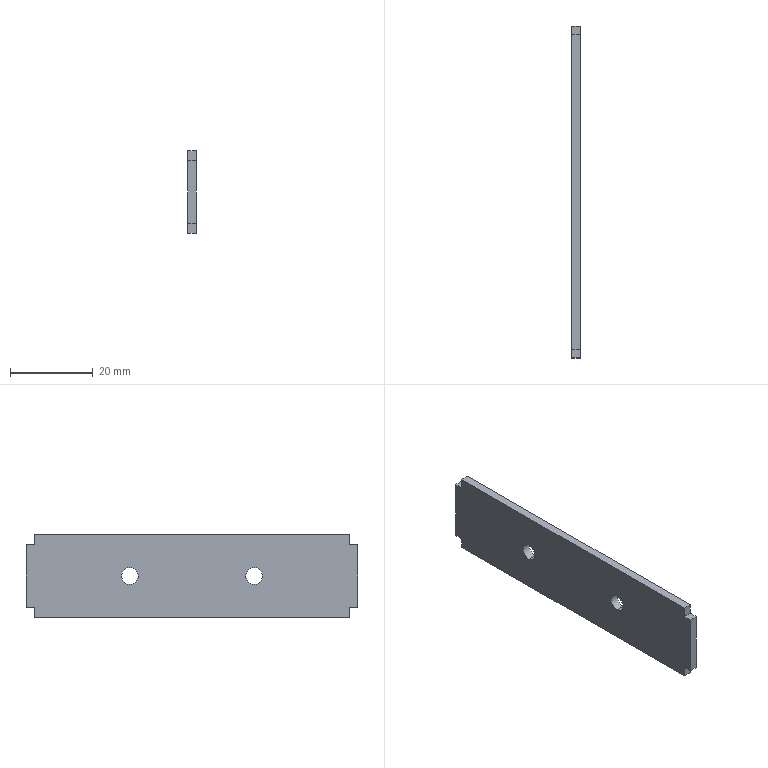Part | STEP file | 1 solid | 18 faces | box 2 x 80 x 20 mm | volume 3110 mm3 | plane 14 | cylinder 4 | commonest cylinder face diameters 4 x4
STEP:
#1=CARTESIAN_POINT('',(0.,0.,0.));
#2=DIRECTION('',(0.,0.,1.));
#3=DIRECTION('',(1.,0.,0.));
#4=AXIS2_PLACEMENT_3D('',#1,#2,#3);
#5=CARTESIAN_POINT('',(0.,-15.,-2.));
#6=VERTEX_POINT('',#5);
#7=CARTESIAN_POINT('',(2.,-15.,-2.));
#8=VERTEX_POINT('',#7);
#9=CARTESIAN_POINT('',(0.,-15.,-2.));
#10=DIRECTION('',(1.,0.,0.));
#11=VECTOR('',#10,1.);
#12=LINE('',#9,#11);
#13=CARTESIAN_POINT('',(0.,-15.,0.));
#14=DIRECTION('',(1.,0.,0.));
#15=DIRECTION('',(0.,0.,-1.));
#16=AXIS2_PLACEMENT_3D('',#13,#14,#15);
#17=CYLINDRICAL_SURFACE('',#16,2.);
#18=CARTESIAN_POINT('',(6.283,0.));
#19=DIRECTION('',(0.,1.));
#20=VECTOR('',#19,1.);
#21=LINE('',#18,#20);
#22=(GEOMETRIC_REPRESENTATION_CONTEXT(2)PARAMETRIC_REPRESENTATION_CONTEXT()REPRESENTATION_CONTEXT('',''));
#23=DEFINITIONAL_REPRESENTATION('',(#21),#22);
#24=PCURVE('',#17,#23);
#25=CARTESIAN_POINT('',(0.,-15.,0.));
#26=DIRECTION('',(1.,0.,0.));
#27=DIRECTION('',(0.,0.,-1.));
#28=AXIS2_PLACEMENT_3D('',#25,#26,#27);
#29=CYLINDRICAL_SURFACE('',#28,2.);
#30=CARTESIAN_POINT('',(0.,0.));
#31=DIRECTION('',(0.,1.));
#32=VECTOR('',#31,1.);
#33=LINE('',#30,#32);
#34=(GEOMETRIC_REPRESENTATION_CONTEXT(2)PARAMETRIC_REPRESENTATION_CONTEXT()REPRESENTATION_CONTEXT('',''));
#35=DEFINITIONAL_REPRESENTATION('',(#33),#34);
#36=PCURVE('',#29,#35);
#37=SURFACE_CURVE('',#12,(#24,#36),.PCURVE_S1.);
#38=EDGE_CURVE('',#6,#8,#37,.T.);
#39=ORIENTED_EDGE('',*,*,#38,.T.);
#40=CARTESIAN_POINT('',(2.,-15.,2.));
#41=VERTEX_POINT('',#40);
#42=CARTESIAN_POINT('',(2.,-15.,0.));
#43=DIRECTION('',(-1.,0.,0.));
#44=DIRECTION('',(0.,0.,-1.));
#45=AXIS2_PLACEMENT_3D('',#42,#43,#44);
#46=CIRCLE('',#45,2.);
#47=CARTESIAN_POINT('',(6.283,2.));
#48=DIRECTION('',(-1.,0.));
#49=VECTOR('',#48,1.);
#50=LINE('',#47,#49);
#51=(GEOMETRIC_REPRESENTATION_CONTEXT(2)PARAMETRIC_REPRESENTATION_CONTEXT()REPRESENTATION_CONTEXT('',''));
#52=DEFINITIONAL_REPRESENTATION('',(#50),#51);
#53=PCURVE('',#17,#52);
#54=CARTESIAN_POINT('',(2.,-19.917,0.));
#55=DIRECTION('',(1.,0.,0.));
#56=DIRECTION('',(0.,0.,-1.));
#57=AXIS2_PLACEMENT_3D('',#54,#55,#56);
#58=PLANE('',#57);
#59=CARTESIAN_POINT('',(2.,4.917));
#60=CARTESIAN_POINT('',(2.,1.453));
#61=CARTESIAN_POINT('',(-1.,3.185));
#62=CARTESIAN_POINT('',(-4.,4.917));
#63=CARTESIAN_POINT('',(-1.,6.649));
#64=CARTESIAN_POINT('',(2.,8.381));
#65=CARTESIAN_POINT('',(2.,4.917));
#66=(BOUNDED_CURVE()B_SPLINE_CURVE(2,(#59,#60,#61,#62,#63,#64,#65),.UNSPECIFIED.,.T.,.F.)B_SPLINE_CURVE_WITH_KNOTS((1,2,2,2,2,1),(-2.094,0.,2.094,4.189,6.283,8.378),.UNSPECIFIED.)CURVE()GEOMETRIC_REPRESENTATION_ITEM()RATIONAL_B_SPLINE_CURVE((1.,0.5,1.,0.5,1.,0.5,1.))REPRESENTATION_ITEM(''));
#67=(GEOMETRIC_REPRESENTATION_CONTEXT(2)PARAMETRIC_REPRESENTATION_CONTEXT()REPRESENTATION_CONTEXT('',''));
#68=DEFINITIONAL_REPRESENTATION('',(#66),#67);
#69=PCURVE('',#58,#68);
#70=SURFACE_CURVE('',#46,(#53,#69),.PCURVE_S1.);
#71=EDGE_CURVE('',#8,#41,#70,.T.);
#72=ORIENTED_EDGE('',*,*,#71,.T.);
#73=CARTESIAN_POINT('',(0.,-15.,2.));
#74=VERTEX_POINT('',#73);
#75=CARTESIAN_POINT('',(0.,-15.,2.));
#76=DIRECTION('',(1.,0.,0.));
#77=VECTOR('',#76,1.);
#78=LINE('',#75,#77);
#79=CARTESIAN_POINT('',(3.142,0.));
#80=DIRECTION('',(0.,1.));
#81=VECTOR('',#80,1.);
#82=LINE('',#79,#81);
#83=(GEOMETRIC_REPRESENTATION_CONTEXT(2)PARAMETRIC_REPRESENTATION_CONTEXT()REPRESENTATION_CONTEXT('',''));
#84=DEFINITIONAL_REPRESENTATION('',(#82),#83);
#85=PCURVE('',#17,#84);
#86=CARTESIAN_POINT('',(3.142,0.));
#87=DIRECTION('',(0.,1.));
#88=VECTOR('',#87,1.);
#89=LINE('',#86,#88);
#90=(GEOMETRIC_REPRESENTATION_CONTEXT(2)PARAMETRIC_REPRESENTATION_CONTEXT()REPRESENTATION_CONTEXT('',''));
#91=DEFINITIONAL_REPRESENTATION('',(#89),#90);
#92=PCURVE('',#29,#91);
#93=SURFACE_CURVE('',#78,(#85,#92),.PCURVE_S1.);
#94=EDGE_CURVE('',#74,#41,#93,.T.);
#95=ORIENTED_EDGE('',*,*,#94,.F.);
#96=CARTESIAN_POINT('',(0.,-15.,0.));
#97=DIRECTION('',(1.,0.,0.));
#98=DIRECTION('',(0.,0.,-1.));
#99=AXIS2_PLACEMENT_3D('',#96,#97,#98);
#100=CIRCLE('',#99,2.);
#101=CARTESIAN_POINT('',(0.,0.));
#102=DIRECTION('',(1.,0.));
#103=VECTOR('',#102,1.);
#104=LINE('',#101,#103);
#105=(GEOMETRIC_REPRESENTATION_CONTEXT(2)PARAMETRIC_REPRESENTATION_CONTEXT()REPRESENTATION_CONTEXT('',''));
#106=DEFINITIONAL_REPRESENTATION('',(#104),#105);
#107=PCURVE('',#17,#106);
#108=CARTESIAN_POINT('',(0.,-19.917,0.));
#109=DIRECTION('',(1.,0.,0.));
#110=DIRECTION('',(0.,0.,-1.));
#111=AXIS2_PLACEMENT_3D('',#108,#109,#110);
#112=PLANE('',#111);
#113=CARTESIAN_POINT('',(0.,4.917));
#114=DIRECTION('',(1.,0.));
#115=AXIS2_PLACEMENT_2D('',#113,#114);
#116=CIRCLE('',#115,2.);
#117=(GEOMETRIC_REPRESENTATION_CONTEXT(2)PARAMETRIC_REPRESENTATION_CONTEXT()REPRESENTATION_CONTEXT('',''));
#118=DEFINITIONAL_REPRESENTATION('',(#116),#117);
#119=PCURVE('',#112,#118);
#120=SURFACE_CURVE('',#100,(#107,#119),.PCURVE_S1.);
#121=EDGE_CURVE('',#74,#6,#120,.T.);
#122=ORIENTED_EDGE('',*,*,#121,.T.);
#123=EDGE_LOOP('',(#39,#72,#95,#122));
#124=FACE_BOUND('',#123,.F.);
#125=ADVANCED_FACE('',(#124),#17,.F.);
#126=CARTESIAN_POINT('',(0.,15.,-2.));
#127=VERTEX_POINT('',#126);
#128=CARTESIAN_POINT('',(2.,15.,-2.));
#129=VERTEX_POINT('',#128);
#130=CARTESIAN_POINT('',(0.,15.,-2.));
#131=DIRECTION('',(1.,0.,0.));
#132=VECTOR('',#131,1.);
#133=LINE('',#130,#132);
#134=CARTESIAN_POINT('',(0.,15.,0.));
#135=DIRECTION('',(1.,0.,0.));
#136=DIRECTION('',(0.,0.,-1.));
#137=AXIS2_PLACEMENT_3D('',#134,#135,#136);
#138=CYLINDRICAL_SURFACE('',#137,2.);
#139=CARTESIAN_POINT('',(6.283,0.));
#140=DIRECTION('',(0.,1.));
#141=VECTOR('',#140,1.);
#142=LINE('',#139,#141);
#143=(GEOMETRIC_REPRESENTATION_CONTEXT(2)PARAMETRIC_REPRESENTATION_CONTEXT()REPRESENTATION_CONTEXT('',''));
#144=DEFINITIONAL_REPRESENTATION('',(#142),#143);
#145=PCURVE('',#138,#144);
#146=CARTESIAN_POINT('',(0.,15.,0.));
#147=DIRECTION('',(1.,0.,0.));
#148=DIRECTION('',(0.,0.,-1.));
#149=AXIS2_PLACEMENT_3D('',#146,#147,#148);
#150=CYLINDRICAL_SURFACE('',#149,2.);
#151=CARTESIAN_POINT('',(0.,0.));
#152=DIRECTION('',(0.,1.));
#153=VECTOR('',#152,1.);
#154=LINE('',#151,#153);
#155=(GEOMETRIC_REPRESENTATION_CONTEXT(2)PARAMETRIC_REPRESENTATION_CONTEXT()REPRESENTATION_CONTEXT('',''));
#156=DEFINITIONAL_REPRESENTATION('',(#154),#155);
#157=PCURVE('',#150,#156);
#158=SURFACE_CURVE('',#133,(#145,#157),.PCURVE_S1.);
#159=EDGE_CURVE('',#127,#129,#158,.T.);
#160=ORIENTED_EDGE('',*,*,#159,.T.);
#161=CARTESIAN_POINT('',(2.,15.,2.));
#162=VERTEX_POINT('',#161);
#163=CARTESIAN_POINT('',(2.,15.,0.));
#164=DIRECTION('',(-1.,0.,0.));
#165=DIRECTION('',(0.,0.,-1.));
#166=AXIS2_PLACEMENT_3D('',#163,#164,#165);
#167=CIRCLE('',#166,2.);
#168=CARTESIAN_POINT('',(6.283,2.));
#169=DIRECTION('',(-1.,0.));
#170=VECTOR('',#169,1.);
#171=LINE('',#168,#170);
#172=(GEOMETRIC_REPRESENTATION_CONTEXT(2)PARAMETRIC_REPRESENTATION_CONTEXT()REPRESENTATION_CONTEXT('',''));
#173=DEFINITIONAL_REPRESENTATION('',(#171),#172);
#174=PCURVE('',#138,#173);
#175=CARTESIAN_POINT('',(2.,34.917));
#176=CARTESIAN_POINT('',(2.,31.453));
#177=CARTESIAN_POINT('',(-1.,33.185));
#178=CARTESIAN_POINT('',(-4.,34.917));
#179=CARTESIAN_POINT('',(-1.,36.649));
#180=CARTESIAN_POINT('',(2.,38.381));
#181=CARTESIAN_POINT('',(2.,34.917));
#182=(BOUNDED_CURVE()B_SPLINE_CURVE(2,(#175,#176,#177,#178,#179,#180,#181),.UNSPECIFIED.,.T.,.F.)B_SPLINE_CURVE_WITH_KNOTS((1,2,2,2,2,1),(-2.094,0.,2.094,4.189,6.283,8.378),.UNSPECIFIED.)CURVE()GEOMETRIC_REPRESENTATION_ITEM()RATIONAL_B_SPLINE_CURVE((1.,0.5,1.,0.5,1.,0.5,1.))REPRESENTATION_ITEM(''));
#183=(GEOMETRIC_REPRESENTATION_CONTEXT(2)PARAMETRIC_REPRESENTATION_CONTEXT()REPRESENTATION_CONTEXT('',''));
#184=DEFINITIONAL_REPRESENTATION('',(#182),#183);
#185=PCURVE('',#58,#184);
#186=SURFACE_CURVE('',#167,(#174,#185),.PCURVE_S1.);
#187=EDGE_CURVE('',#129,#162,#186,.T.);
#188=ORIENTED_EDGE('',*,*,#187,.T.);
#189=CARTESIAN_POINT('',(0.,15.,2.));
#190=VERTEX_POINT('',#189);
#191=CARTESIAN_POINT('',(0.,15.,2.));
#192=DIRECTION('',(1.,0.,0.));
#193=VECTOR('',#192,1.);
#194=LINE('',#191,#193);
#195=CARTESIAN_POINT('',(3.142,0.));
#196=DIRECTION('',(0.,1.));
#197=VECTOR('',#196,1.);
#198=LINE('',#195,#197);
#199=(GEOMETRIC_REPRESENTATION_CONTEXT(2)PARAMETRIC_REPRESENTATION_CONTEXT()REPRESENTATION_CONTEXT('',''));
#200=DEFINITIONAL_REPRESENTATION('',(#198),#199);
#201=PCURVE('',#138,#200);
#202=CARTESIAN_POINT('',(3.142,0.));
#203=DIRECTION('',(0.,1.));
#204=VECTOR('',#203,1.);
#205=LINE('',#202,#204);
#206=(GEOMETRIC_REPRESENTATION_CONTEXT(2)PARAMETRIC_REPRESENTATION_CONTEXT()REPRESENTATION_CONTEXT('',''));
#207=DEFINITIONAL_REPRESENTATION('',(#205),#206);
#208=PCURVE('',#150,#207);
#209=SURFACE_CURVE('',#194,(#201,#208),.PCURVE_S1.);
#210=EDGE_CURVE('',#190,#162,#209,.T.);
#211=ORIENTED_EDGE('',*,*,#210,.F.);
#212=CARTESIAN_POINT('',(0.,15.,0.));
#213=DIRECTION('',(1.,0.,0.));
#214=DIRECTION('',(0.,0.,-1.));
#215=AXIS2_PLACEMENT_3D('',#212,#213,#214);
#216=CIRCLE('',#215,2.);
#217=CARTESIAN_POINT('',(0.,0.));
#218=DIRECTION('',(1.,0.));
#219=VECTOR('',#218,1.);
#220=LINE('',#217,#219);
#221=(GEOMETRIC_REPRESENTATION_CONTEXT(2)PARAMETRIC_REPRESENTATION_CONTEXT()REPRESENTATION_CONTEXT('',''));
#222=DEFINITIONAL_REPRESENTATION('',(#220),#221);
#223=PCURVE('',#138,#222);
#224=CARTESIAN_POINT('',(0.,34.917));
#225=DIRECTION('',(1.,0.));
#226=AXIS2_PLACEMENT_2D('',#224,#225);
#227=CIRCLE('',#226,2.);
#228=(GEOMETRIC_REPRESENTATION_CONTEXT(2)PARAMETRIC_REPRESENTATION_CONTEXT()REPRESENTATION_CONTEXT('',''));
#229=DEFINITIONAL_REPRESENTATION('',(#227),#228);
#230=PCURVE('',#112,#229);
#231=SURFACE_CURVE('',#216,(#223,#230),.PCURVE_S1.);
#232=EDGE_CURVE('',#190,#127,#231,.T.);
#233=ORIENTED_EDGE('',*,*,#232,.T.);
#234=EDGE_LOOP('',(#160,#188,#211,#233));
#235=FACE_BOUND('',#234,.F.);
#236=ADVANCED_FACE('',(#235),#138,.F.);
#237=CARTESIAN_POINT('',(2.,40.,7.5));
#238=VERTEX_POINT('',#237);
#239=CARTESIAN_POINT('',(2.,38.,7.5));
#240=VERTEX_POINT('',#239);
#241=CARTESIAN_POINT('',(2.,-19.917,7.5));
#242=DIRECTION('',(0.,-1.,0.));
#243=VECTOR('',#242,1.);
#244=LINE('',#241,#243);
#245=CARTESIAN_POINT('',(-7.5,0.));
#246=DIRECTION('',(0.,-1.));
#247=VECTOR('',#246,1.);
#248=LINE('',#245,#247);
#249=(GEOMETRIC_REPRESENTATION_CONTEXT(2)PARAMETRIC_REPRESENTATION_CONTEXT()REPRESENTATION_CONTEXT('',''));
#250=DEFINITIONAL_REPRESENTATION('',(#248),#249);
#251=PCURVE('',#58,#250);
#252=CARTESIAN_POINT('',(0.,40.,7.5));
#253=DIRECTION('',(0.,0.,1.));
#254=DIRECTION('',(0.,-1.,0.));
#255=AXIS2_PLACEMENT_3D('',#252,#253,#254);
#256=PLANE('',#255);
#257=CARTESIAN_POINT('',(59.917,2.));
#258=DIRECTION('',(1.,0.));
#259=VECTOR('',#258,1.);
#260=LINE('',#257,#259);
#261=(GEOMETRIC_REPRESENTATION_CONTEXT(2)PARAMETRIC_REPRESENTATION_CONTEXT()REPRESENTATION_CONTEXT('',''));
#262=DEFINITIONAL_REPRESENTATION('',(#260),#261);
#263=PCURVE('',#256,#262);
#264=SURFACE_CURVE('',#244,(#251,#263),.PCURVE_S1.);
#265=EDGE_CURVE('',#238,#240,#264,.T.);
#266=ORIENTED_EDGE('',*,*,#265,.T.);
#267=CARTESIAN_POINT('',(2.,38.,10.));
#268=VERTEX_POINT('',#267);
#269=CARTESIAN_POINT('',(2.,38.,0.));
#270=DIRECTION('',(0.,0.,1.));
#271=VECTOR('',#270,1.);
#272=LINE('',#269,#271);
#273=CARTESIAN_POINT('',(0.,57.917));
#274=DIRECTION('',(-1.,0.));
#275=VECTOR('',#274,1.);
#276=LINE('',#273,#275);
#277=(GEOMETRIC_REPRESENTATION_CONTEXT(2)PARAMETRIC_REPRESENTATION_CONTEXT()REPRESENTATION_CONTEXT('',''));
#278=DEFINITIONAL_REPRESENTATION('',(#276),#277);
#279=PCURVE('',#58,#278);
#280=CARTESIAN_POINT('',(0.,38.,7.5));
#281=DIRECTION('',(0.,1.,0.));
#282=DIRECTION('',(0.,0.,1.));
#283=AXIS2_PLACEMENT_3D('',#280,#281,#282);
#284=PLANE('',#283);
#285=CARTESIAN_POINT('',(-7.5,2.));
#286=DIRECTION('',(1.,0.));
#287=VECTOR('',#286,1.);
#288=LINE('',#285,#287);
#289=(GEOMETRIC_REPRESENTATION_CONTEXT(2)PARAMETRIC_REPRESENTATION_CONTEXT()REPRESENTATION_CONTEXT('',''));
#290=DEFINITIONAL_REPRESENTATION('',(#288),#289);
#291=PCURVE('',#284,#290);
#292=SURFACE_CURVE('',#272,(#279,#291),.PCURVE_S1.);
#293=EDGE_CURVE('',#240,#268,#292,.T.);
#294=ORIENTED_EDGE('',*,*,#293,.T.);
#295=CARTESIAN_POINT('',(2.,-38.,10.));
#296=VERTEX_POINT('',#295);
#297=CARTESIAN_POINT('',(2.,-19.917,10.));
#298=DIRECTION('',(0.,-1.,0.));
#299=VECTOR('',#298,1.);
#300=LINE('',#297,#299);
#301=CARTESIAN_POINT('',(-10.,0.));
#302=DIRECTION('',(0.,-1.));
#303=VECTOR('',#302,1.);
#304=LINE('',#301,#303);
#305=(GEOMETRIC_REPRESENTATION_CONTEXT(2)PARAMETRIC_REPRESENTATION_CONTEXT()REPRESENTATION_CONTEXT('',''));
#306=DEFINITIONAL_REPRESENTATION('',(#304),#305);
#307=PCURVE('',#58,#306);
#308=CARTESIAN_POINT('',(0.,0.,10.));
#309=DIRECTION('',(0.,0.,1.));
#310=DIRECTION('',(1.,0.,0.));
#311=AXIS2_PLACEMENT_3D('',#308,#309,#310);
#312=PLANE('',#311);
#313=CARTESIAN_POINT('',(2.,-19.917));
#314=DIRECTION('',(0.,-1.));
#315=VECTOR('',#314,1.);
#316=LINE('',#313,#315);
#317=(GEOMETRIC_REPRESENTATION_CONTEXT(2)PARAMETRIC_REPRESENTATION_CONTEXT()REPRESENTATION_CONTEXT('',''));
#318=DEFINITIONAL_REPRESENTATION('',(#316),#317);
#319=PCURVE('',#312,#318);
#320=SURFACE_CURVE('',#300,(#307,#319),.PCURVE_S1.);
#321=EDGE_CURVE('',#268,#296,#320,.T.);
#322=ORIENTED_EDGE('',*,*,#321,.T.);
#323=CARTESIAN_POINT('',(2.,-38.,7.5));
#324=VERTEX_POINT('',#323);
#325=CARTESIAN_POINT('',(2.,-38.,0.));
#326=DIRECTION('',(0.,0.,-1.));
#327=VECTOR('',#326,1.);
#328=LINE('',#325,#327);
#329=CARTESIAN_POINT('',(0.,-18.083));
#330=DIRECTION('',(1.,0.));
#331=VECTOR('',#330,1.);
#332=LINE('',#329,#331);
#333=(GEOMETRIC_REPRESENTATION_CONTEXT(2)PARAMETRIC_REPRESENTATION_CONTEXT()REPRESENTATION_CONTEXT('',''));
#334=DEFINITIONAL_REPRESENTATION('',(#332),#333);
#335=PCURVE('',#58,#334);
#336=CARTESIAN_POINT('',(0.,-38.,10.));
#337=DIRECTION('',(0.,-1.,0.));
#338=DIRECTION('',(0.,0.,-1.));
#339=AXIS2_PLACEMENT_3D('',#336,#337,#338);
#340=PLANE('',#339);
#341=CARTESIAN_POINT('',(10.,2.));
#342=DIRECTION('',(1.,0.));
#343=VECTOR('',#342,1.);
#344=LINE('',#341,#343);
#345=(GEOMETRIC_REPRESENTATION_CONTEXT(2)PARAMETRIC_REPRESENTATION_CONTEXT()REPRESENTATION_CONTEXT('',''));
#346=DEFINITIONAL_REPRESENTATION('',(#344),#345);
#347=PCURVE('',#340,#346);
#348=SURFACE_CURVE('',#328,(#335,#347),.PCURVE_S1.);
#349=EDGE_CURVE('',#296,#324,#348,.T.);
#350=ORIENTED_EDGE('',*,*,#349,.T.);
#351=CARTESIAN_POINT('',(2.,-40.,7.5));
#352=VERTEX_POINT('',#351);
#353=CARTESIAN_POINT('',(2.,-19.917,7.5));
#354=DIRECTION('',(0.,-1.,0.));
#355=VECTOR('',#354,1.);
#356=LINE('',#353,#355);
#357=CARTESIAN_POINT('',(-7.5,0.));
#358=DIRECTION('',(0.,-1.));
#359=VECTOR('',#358,1.);
#360=LINE('',#357,#359);
#361=(GEOMETRIC_REPRESENTATION_CONTEXT(2)PARAMETRIC_REPRESENTATION_CONTEXT()REPRESENTATION_CONTEXT('',''));
#362=DEFINITIONAL_REPRESENTATION('',(#360),#361);
#363=PCURVE('',#58,#362);
#364=CARTESIAN_POINT('',(0.,-38.,7.5));
#365=DIRECTION('',(0.,0.,1.));
#366=DIRECTION('',(1.,0.,0.));
#367=AXIS2_PLACEMENT_3D('',#364,#365,#366);
#368=PLANE('',#367);
#369=CARTESIAN_POINT('',(2.,18.083));
#370=DIRECTION('',(0.,-1.));
#371=VECTOR('',#370,1.);
#372=LINE('',#369,#371);
#373=(GEOMETRIC_REPRESENTATION_CONTEXT(2)PARAMETRIC_REPRESENTATION_CONTEXT()REPRESENTATION_CONTEXT('',''));
#374=DEFINITIONAL_REPRESENTATION('',(#372),#373);
#375=PCURVE('',#368,#374);
#376=SURFACE_CURVE('',#356,(#363,#375),.PCURVE_S1.);
#377=EDGE_CURVE('',#324,#352,#376,.T.);
#378=ORIENTED_EDGE('',*,*,#377,.T.);
#379=CARTESIAN_POINT('',(2.,-40.,-7.5));
#380=VERTEX_POINT('',#379);
#381=CARTESIAN_POINT('',(2.,-40.,0.));
#382=DIRECTION('',(0.,0.,-1.));
#383=VECTOR('',#382,1.);
#384=LINE('',#381,#383);
#385=CARTESIAN_POINT('',(0.,-20.083));
#386=DIRECTION('',(1.,0.));
#387=VECTOR('',#386,1.);
#388=LINE('',#385,#387);
#389=(GEOMETRIC_REPRESENTATION_CONTEXT(2)PARAMETRIC_REPRESENTATION_CONTEXT()REPRESENTATION_CONTEXT('',''));
#390=DEFINITIONAL_REPRESENTATION('',(#388),#389);
#391=PCURVE('',#58,#390);
#392=CARTESIAN_POINT('',(0.,-40.,7.5));
#393=DIRECTION('',(0.,-1.,0.));
#394=DIRECTION('',(0.,0.,-1.));
#395=AXIS2_PLACEMENT_3D('',#392,#393,#394);
#396=PLANE('',#395);
#397=CARTESIAN_POINT('',(7.5,2.));
#398=DIRECTION('',(1.,0.));
#399=VECTOR('',#398,1.);
#400=LINE('',#397,#399);
#401=(GEOMETRIC_REPRESENTATION_CONTEXT(2)PARAMETRIC_REPRESENTATION_CONTEXT()REPRESENTATION_CONTEXT('',''));
#402=DEFINITIONAL_REPRESENTATION('',(#400),#401);
#403=PCURVE('',#396,#402);
#404=SURFACE_CURVE('',#384,(#391,#403),.PCURVE_S1.);
#405=EDGE_CURVE('',#352,#380,#404,.T.);
#406=ORIENTED_EDGE('',*,*,#405,.T.);
#407=CARTESIAN_POINT('',(2.,-38.,-7.5));
#408=VERTEX_POINT('',#407);
#409=CARTESIAN_POINT('',(2.,-19.917,-7.5));
#410=DIRECTION('',(0.,1.,0.));
#411=VECTOR('',#410,1.);
#412=LINE('',#409,#411);
#413=CARTESIAN_POINT('',(7.5,0.));
#414=DIRECTION('',(0.,1.));
#415=VECTOR('',#414,1.);
#416=LINE('',#413,#415);
#417=(GEOMETRIC_REPRESENTATION_CONTEXT(2)PARAMETRIC_REPRESENTATION_CONTEXT()REPRESENTATION_CONTEXT('',''));
#418=DEFINITIONAL_REPRESENTATION('',(#416),#417);
#419=PCURVE('',#58,#418);
#420=CARTESIAN_POINT('',(0.,-40.,-7.5));
#421=DIRECTION('',(0.,0.,-1.));
#422=DIRECTION('',(-1.,0.,0.));
#423=AXIS2_PLACEMENT_3D('',#420,#421,#422);
#424=PLANE('',#423);
#425=CARTESIAN_POINT('',(-2.,20.083));
#426=DIRECTION('',(0.,1.));
#427=VECTOR('',#426,1.);
#428=LINE('',#425,#427);
#429=(GEOMETRIC_REPRESENTATION_CONTEXT(2)PARAMETRIC_REPRESENTATION_CONTEXT()REPRESENTATION_CONTEXT('',''));
#430=DEFINITIONAL_REPRESENTATION('',(#428),#429);
#431=PCURVE('',#424,#430);
#432=SURFACE_CURVE('',#412,(#419,#431),.PCURVE_S1.);
#433=EDGE_CURVE('',#380,#408,#432,.T.);
#434=ORIENTED_EDGE('',*,*,#433,.T.);
#435=CARTESIAN_POINT('',(2.,-38.,-10.));
#436=VERTEX_POINT('',#435);
#437=CARTESIAN_POINT('',(2.,-38.,0.));
#438=DIRECTION('',(0.,0.,-1.));
#439=VECTOR('',#438,1.);
#440=LINE('',#437,#439);
#441=CARTESIAN_POINT('',(0.,-18.083));
#442=DIRECTION('',(1.,0.));
#443=VECTOR('',#442,1.);
#444=LINE('',#441,#443);
#445=(GEOMETRIC_REPRESENTATION_CONTEXT(2)PARAMETRIC_REPRESENTATION_CONTEXT()REPRESENTATION_CONTEXT('',''));
#446=DEFINITIONAL_REPRESENTATION('',(#444),#445);
#447=PCURVE('',#58,#446);
#448=CARTESIAN_POINT('',(0.,-38.,-7.5));
#449=DIRECTION('',(0.,-1.,0.));
#450=DIRECTION('',(0.,0.,-1.));
#451=AXIS2_PLACEMENT_3D('',#448,#449,#450);
#452=PLANE('',#451);
#453=CARTESIAN_POINT('',(-7.5,2.));
#454=DIRECTION('',(1.,0.));
#455=VECTOR('',#454,1.);
#456=LINE('',#453,#455);
#457=(GEOMETRIC_REPRESENTATION_CONTEXT(2)PARAMETRIC_REPRESENTATION_CONTEXT()REPRESENTATION_CONTEXT('',''));
#458=DEFINITIONAL_REPRESENTATION('',(#456),#457);
#459=PCURVE('',#452,#458);
#460=SURFACE_CURVE('',#440,(#447,#459),.PCURVE_S1.);
#461=EDGE_CURVE('',#408,#436,#460,.T.);
#462=ORIENTED_EDGE('',*,*,#461,.T.);
#463=CARTESIAN_POINT('',(2.,38.,-10.));
#464=VERTEX_POINT('',#463);
#465=CARTESIAN_POINT('',(2.,-19.917,-10.));
#466=DIRECTION('',(0.,1.,0.));
#467=VECTOR('',#466,1.);
#468=LINE('',#465,#467);
#469=CARTESIAN_POINT('',(10.,0.));
#470=DIRECTION('',(0.,1.));
#471=VECTOR('',#470,1.);
#472=LINE('',#469,#471);
#473=(GEOMETRIC_REPRESENTATION_CONTEXT(2)PARAMETRIC_REPRESENTATION_CONTEXT()REPRESENTATION_CONTEXT('',''));
#474=DEFINITIONAL_REPRESENTATION('',(#472),#473);
#475=PCURVE('',#58,#474);
#476=CARTESIAN_POINT('',(0.,-38.,-10.));
#477=DIRECTION('',(0.,0.,-1.));
#478=DIRECTION('',(-1.,0.,0.));
#479=AXIS2_PLACEMENT_3D('',#476,#477,#478);
#480=PLANE('',#479);
#481=CARTESIAN_POINT('',(-2.,18.083));
#482=DIRECTION('',(0.,1.));
#483=VECTOR('',#482,1.);
#484=LINE('',#481,#483);
#485=(GEOMETRIC_REPRESENTATION_CONTEXT(2)PARAMETRIC_REPRESENTATION_CONTEXT()REPRESENTATION_CONTEXT('',''));
#486=DEFINITIONAL_REPRESENTATION('',(#484),#485);
#487=PCURVE('',#480,#486);
#488=SURFACE_CURVE('',#468,(#475,#487),.PCURVE_S1.);
#489=EDGE_CURVE('',#436,#464,#488,.T.);
#490=ORIENTED_EDGE('',*,*,#489,.T.);
#491=CARTESIAN_POINT('',(2.,38.,-7.5));
#492=VERTEX_POINT('',#491);
#493=CARTESIAN_POINT('',(2.,38.,0.));
#494=DIRECTION('',(0.,0.,1.));
#495=VECTOR('',#494,1.);
#496=LINE('',#493,#495);
#497=CARTESIAN_POINT('',(0.,57.917));
#498=DIRECTION('',(-1.,0.));
#499=VECTOR('',#498,1.);
#500=LINE('',#497,#499);
#501=(GEOMETRIC_REPRESENTATION_CONTEXT(2)PARAMETRIC_REPRESENTATION_CONTEXT()REPRESENTATION_CONTEXT('',''));
#502=DEFINITIONAL_REPRESENTATION('',(#500),#501);
#503=PCURVE('',#58,#502);
#504=CARTESIAN_POINT('',(0.,38.,-10.));
#505=DIRECTION('',(0.,1.,0.));
#506=DIRECTION('',(0.,0.,1.));
#507=AXIS2_PLACEMENT_3D('',#504,#505,#506);
#508=PLANE('',#507);
#509=CARTESIAN_POINT('',(10.,2.));
#510=DIRECTION('',(1.,0.));
#511=VECTOR('',#510,1.);
#512=LINE('',#509,#511);
#513=(GEOMETRIC_REPRESENTATION_CONTEXT(2)PARAMETRIC_REPRESENTATION_CONTEXT()REPRESENTATION_CONTEXT('',''));
#514=DEFINITIONAL_REPRESENTATION('',(#512),#513);
#515=PCURVE('',#508,#514);
#516=SURFACE_CURVE('',#496,(#503,#515),.PCURVE_S1.);
#517=EDGE_CURVE('',#464,#492,#516,.T.);
#518=ORIENTED_EDGE('',*,*,#517,.T.);
#519=CARTESIAN_POINT('',(2.,40.,-7.5));
#520=VERTEX_POINT('',#519);
#521=CARTESIAN_POINT('',(2.,-19.917,-7.5));
#522=DIRECTION('',(0.,1.,0.));
#523=VECTOR('',#522,1.);
#524=LINE('',#521,#523);
#525=CARTESIAN_POINT('',(7.5,0.));
#526=DIRECTION('',(0.,1.));
#527=VECTOR('',#526,1.);
#528=LINE('',#525,#527);
#529=(GEOMETRIC_REPRESENTATION_CONTEXT(2)PARAMETRIC_REPRESENTATION_CONTEXT()REPRESENTATION_CONTEXT('',''));
#530=DEFINITIONAL_REPRESENTATION('',(#528),#529);
#531=PCURVE('',#58,#530);
#532=CARTESIAN_POINT('',(0.,38.,-7.5));
#533=DIRECTION('',(0.,0.,-1.));
#534=DIRECTION('',(0.,1.,0.));
#535=AXIS2_PLACEMENT_3D('',#532,#533,#534);
#536=PLANE('',#535);
#537=CARTESIAN_POINT('',(-57.917,2.));
#538=DIRECTION('',(1.,0.));
#539=VECTOR('',#538,1.);
#540=LINE('',#537,#539);
#541=(GEOMETRIC_REPRESENTATION_CONTEXT(2)PARAMETRIC_REPRESENTATION_CONTEXT()REPRESENTATION_CONTEXT('',''));
#542=DEFINITIONAL_REPRESENTATION('',(#540),#541);
#543=PCURVE('',#536,#542);
#544=SURFACE_CURVE('',#524,(#531,#543),.PCURVE_S1.);
#545=EDGE_CURVE('',#492,#520,#544,.T.);
#546=ORIENTED_EDGE('',*,*,#545,.T.);
#547=CARTESIAN_POINT('',(2.,40.,0.));
#548=DIRECTION('',(0.,0.,1.));
#549=VECTOR('',#548,1.);
#550=LINE('',#547,#549);
#551=CARTESIAN_POINT('',(0.,59.917));
#552=DIRECTION('',(-1.,0.));
#553=VECTOR('',#552,1.);
#554=LINE('',#551,#553);
#555=(GEOMETRIC_REPRESENTATION_CONTEXT(2)PARAMETRIC_REPRESENTATION_CONTEXT()REPRESENTATION_CONTEXT('',''));
#556=DEFINITIONAL_REPRESENTATION('',(#554),#555);
#557=PCURVE('',#58,#556);
#558=CARTESIAN_POINT('',(0.,40.,-7.5));
#559=DIRECTION('',(0.,1.,0.));
#560=DIRECTION('',(0.,0.,1.));
#561=AXIS2_PLACEMENT_3D('',#558,#559,#560);
#562=PLANE('',#561);
#563=CARTESIAN_POINT('',(7.5,2.));
#564=DIRECTION('',(1.,0.));
#565=VECTOR('',#564,1.);
#566=LINE('',#563,#565);
#567=(GEOMETRIC_REPRESENTATION_CONTEXT(2)PARAMETRIC_REPRESENTATION_CONTEXT()REPRESENTATION_CONTEXT('',''));
#568=DEFINITIONAL_REPRESENTATION('',(#566),#567);
#569=PCURVE('',#562,#568);
#570=SURFACE_CURVE('',#550,(#557,#569),.PCURVE_S1.);
#571=EDGE_CURVE('',#520,#238,#570,.T.);
#572=ORIENTED_EDGE('',*,*,#571,.T.);
#573=EDGE_LOOP('',(#266,#294,#322,#350,#378,#406,#434,#462,#490,#518,#546,#572));
#574=FACE_BOUND('',#573,.T.);
#575=ORIENTED_EDGE('',*,*,#71,.T.);
#576=CARTESIAN_POINT('',(2.,-15.,0.));
#577=DIRECTION('',(-1.,0.,0.));
#578=DIRECTION('',(0.,0.,-1.));
#579=AXIS2_PLACEMENT_3D('',#576,#577,#578);
#580=CIRCLE('',#579,2.);
#581=CARTESIAN_POINT('',(2.,4.917));
#582=CARTESIAN_POINT('',(2.,1.453));
#583=CARTESIAN_POINT('',(-1.,3.185));
#584=CARTESIAN_POINT('',(-4.,4.917));
#585=CARTESIAN_POINT('',(-1.,6.649));
#586=CARTESIAN_POINT('',(2.,8.381));
#587=CARTESIAN_POINT('',(2.,4.917));
#588=(BOUNDED_CURVE()B_SPLINE_CURVE(2,(#581,#582,#583,#584,#585,#586,#587),.UNSPECIFIED.,.T.,.F.)B_SPLINE_CURVE_WITH_KNOTS((1,2,2,2,2,1),(-2.094,0.,2.094,4.189,6.283,8.378),.UNSPECIFIED.)CURVE()GEOMETRIC_REPRESENTATION_ITEM()RATIONAL_B_SPLINE_CURVE((1.,0.5,1.,0.5,1.,0.5,1.))REPRESENTATION_ITEM(''));
#589=(GEOMETRIC_REPRESENTATION_CONTEXT(2)PARAMETRIC_REPRESENTATION_CONTEXT()REPRESENTATION_CONTEXT('',''));
#590=DEFINITIONAL_REPRESENTATION('',(#588),#589);
#591=PCURVE('',#58,#590);
#592=CARTESIAN_POINT('',(6.283,2.));
#593=DIRECTION('',(-1.,0.));
#594=VECTOR('',#593,1.);
#595=LINE('',#592,#594);
#596=(GEOMETRIC_REPRESENTATION_CONTEXT(2)PARAMETRIC_REPRESENTATION_CONTEXT()REPRESENTATION_CONTEXT('',''));
#597=DEFINITIONAL_REPRESENTATION('',(#595),#596);
#598=PCURVE('',#29,#597);
#599=SURFACE_CURVE('',#580,(#591,#598),.PCURVE_S1.);
#600=EDGE_CURVE('',#41,#8,#599,.T.);
#601=ORIENTED_EDGE('',*,*,#600,.T.);
#602=EDGE_LOOP('',(#575,#601));
#603=FACE_BOUND('',#602,.T.);
#604=ORIENTED_EDGE('',*,*,#187,.T.);
#605=CARTESIAN_POINT('',(2.,15.,0.));
#606=DIRECTION('',(-1.,0.,0.));
#607=DIRECTION('',(0.,0.,-1.));
#608=AXIS2_PLACEMENT_3D('',#605,#606,#607);
#609=CIRCLE('',#608,2.);
#610=CARTESIAN_POINT('',(2.,34.917));
#611=CARTESIAN_POINT('',(2.,31.453));
#612=CARTESIAN_POINT('',(-1.,33.185));
#613=CARTESIAN_POINT('',(-4.,34.917));
#614=CARTESIAN_POINT('',(-1.,36.649));
#615=CARTESIAN_POINT('',(2.,38.381));
#616=CARTESIAN_POINT('',(2.,34.917));
#617=(BOUNDED_CURVE()B_SPLINE_CURVE(2,(#610,#611,#612,#613,#614,#615,#616),.UNSPECIFIED.,.T.,.F.)B_SPLINE_CURVE_WITH_KNOTS((1,2,2,2,2,1),(-2.094,0.,2.094,4.189,6.283,8.378),.UNSPECIFIED.)CURVE()GEOMETRIC_REPRESENTATION_ITEM()RATIONAL_B_SPLINE_CURVE((1.,0.5,1.,0.5,1.,0.5,1.))REPRESENTATION_ITEM(''));
#618=(GEOMETRIC_REPRESENTATION_CONTEXT(2)PARAMETRIC_REPRESENTATION_CONTEXT()REPRESENTATION_CONTEXT('',''));
#619=DEFINITIONAL_REPRESENTATION('',(#617),#618);
#620=PCURVE('',#58,#619);
#621=CARTESIAN_POINT('',(6.283,2.));
#622=DIRECTION('',(-1.,0.));
#623=VECTOR('',#622,1.);
#624=LINE('',#621,#623);
#625=(GEOMETRIC_REPRESENTATION_CONTEXT(2)PARAMETRIC_REPRESENTATION_CONTEXT()REPRESENTATION_CONTEXT('',''));
#626=DEFINITIONAL_REPRESENTATION('',(#624),#625);
#627=PCURVE('',#150,#626);
#628=SURFACE_CURVE('',#609,(#620,#627),.PCURVE_S1.);
#629=EDGE_CURVE('',#162,#129,#628,.T.);
#630=ORIENTED_EDGE('',*,*,#629,.T.);
#631=EDGE_LOOP('',(#604,#630));
#632=FACE_BOUND('',#631,.T.);
#633=ADVANCED_FACE('',(#574,#603,#632),#58,.T.);
#634=ORIENTED_EDGE('',*,*,#293,.F.);
#635=CARTESIAN_POINT('',(0.,38.,7.5));
#636=VERTEX_POINT('',#635);
#637=CARTESIAN_POINT('',(0.,38.,7.5));
#638=DIRECTION('',(-1.,0.,0.));
#639=VECTOR('',#638,1.);
#640=LINE('',#637,#639);
#641=CARTESIAN_POINT('',(0.,0.));
#642=DIRECTION('',(0.,-1.));
#643=VECTOR('',#642,1.);
#644=LINE('',#641,#643);
#645=(GEOMETRIC_REPRESENTATION_CONTEXT(2)PARAMETRIC_REPRESENTATION_CONTEXT()REPRESENTATION_CONTEXT('',''));
#646=DEFINITIONAL_REPRESENTATION('',(#644),#645);
#647=PCURVE('',#284,#646);
#648=CARTESIAN_POINT('',(2.,0.));
#649=DIRECTION('',(0.,-1.));
#650=VECTOR('',#649,1.);
#651=LINE('',#648,#650);
#652=(GEOMETRIC_REPRESENTATION_CONTEXT(2)PARAMETRIC_REPRESENTATION_CONTEXT()REPRESENTATION_CONTEXT('',''));
#653=DEFINITIONAL_REPRESENTATION('',(#651),#652);
#654=PCURVE('',#256,#653);
#655=SURFACE_CURVE('',#640,(#647,#654),.PCURVE_S1.);
#656=EDGE_CURVE('',#240,#636,#655,.T.);
#657=ORIENTED_EDGE('',*,*,#656,.T.);
#658=CARTESIAN_POINT('',(0.,38.,10.));
#659=VERTEX_POINT('',#658);
#660=CARTESIAN_POINT('',(0.,38.,7.5));
#661=DIRECTION('',(0.,0.,1.));
#662=VECTOR('',#661,1.);
#663=LINE('',#660,#662);
#664=CARTESIAN_POINT('',(0.,0.));
#665=DIRECTION('',(1.,0.));
#666=VECTOR('',#665,1.);
#667=LINE('',#664,#666);
#668=(GEOMETRIC_REPRESENTATION_CONTEXT(2)PARAMETRIC_REPRESENTATION_CONTEXT()REPRESENTATION_CONTEXT('',''));
#669=DEFINITIONAL_REPRESENTATION('',(#667),#668);
#670=PCURVE('',#284,#669);
#671=CARTESIAN_POINT('',(-7.5,57.917));
#672=DIRECTION('',(-1.,0.));
#673=VECTOR('',#672,1.);
#674=LINE('',#671,#673);
#675=(GEOMETRIC_REPRESENTATION_CONTEXT(2)PARAMETRIC_REPRESENTATION_CONTEXT()REPRESENTATION_CONTEXT('',''));
#676=DEFINITIONAL_REPRESENTATION('',(#674),#675);
#677=PCURVE('',#112,#676);
#678=SURFACE_CURVE('',#663,(#670,#677),.PCURVE_S1.);
#679=EDGE_CURVE('',#636,#659,#678,.T.);
#680=ORIENTED_EDGE('',*,*,#679,.T.);
#681=CARTESIAN_POINT('',(0.,38.,10.));
#682=DIRECTION('',(1.,0.,0.));
#683=VECTOR('',#682,1.);
#684=LINE('',#681,#683);
#685=CARTESIAN_POINT('',(2.5,0.));
#686=DIRECTION('',(0.,1.));
#687=VECTOR('',#686,1.);
#688=LINE('',#685,#687);
#689=(GEOMETRIC_REPRESENTATION_CONTEXT(2)PARAMETRIC_REPRESENTATION_CONTEXT()REPRESENTATION_CONTEXT('',''));
#690=DEFINITIONAL_REPRESENTATION('',(#688),#689);
#691=PCURVE('',#284,#690);
#692=CARTESIAN_POINT('',(0.,38.));
#693=DIRECTION('',(1.,0.));
#694=VECTOR('',#693,1.);
#695=LINE('',#692,#694);
#696=(GEOMETRIC_REPRESENTATION_CONTEXT(2)PARAMETRIC_REPRESENTATION_CONTEXT()REPRESENTATION_CONTEXT('',''));
#697=DEFINITIONAL_REPRESENTATION('',(#695),#696);
#698=PCURVE('',#312,#697);
#699=SURFACE_CURVE('',#684,(#691,#698),.PCURVE_S1.);
#700=EDGE_CURVE('',#659,#268,#699,.T.);
#701=ORIENTED_EDGE('',*,*,#700,.T.);
#702=EDGE_LOOP('',(#634,#657,#680,#701));
#703=FACE_BOUND('',#702,.T.);
#704=ADVANCED_FACE('',(#703),#284,.T.);
#705=ORIENTED_EDGE('',*,*,#265,.F.);
#706=CARTESIAN_POINT('',(0.,40.,7.5));
#707=VERTEX_POINT('',#706);
#708=CARTESIAN_POINT('',(0.,40.,7.5));
#709=DIRECTION('',(-1.,0.,0.));
#710=VECTOR('',#709,1.);
#711=LINE('',#708,#710);
#712=CARTESIAN_POINT('',(0.,0.));
#713=DIRECTION('',(0.,-1.));
#714=VECTOR('',#713,1.);
#715=LINE('',#712,#714);
#716=(GEOMETRIC_REPRESENTATION_CONTEXT(2)PARAMETRIC_REPRESENTATION_CONTEXT()REPRESENTATION_CONTEXT('',''));
#717=DEFINITIONAL_REPRESENTATION('',(#715),#716);
#718=PCURVE('',#256,#717);
#719=CARTESIAN_POINT('',(15.,0.));
#720=DIRECTION('',(0.,-1.));
#721=VECTOR('',#720,1.);
#722=LINE('',#719,#721);
#723=(GEOMETRIC_REPRESENTATION_CONTEXT(2)PARAMETRIC_REPRESENTATION_CONTEXT()REPRESENTATION_CONTEXT('',''));
#724=DEFINITIONAL_REPRESENTATION('',(#722),#723);
#725=PCURVE('',#562,#724);
#726=SURFACE_CURVE('',#711,(#718,#725),.PCURVE_S1.);
#727=EDGE_CURVE('',#238,#707,#726,.T.);
#728=ORIENTED_EDGE('',*,*,#727,.T.);
#729=CARTESIAN_POINT('',(0.,40.,7.5));
#730=DIRECTION('',(0.,-1.,0.));
#731=VECTOR('',#730,1.);
#732=LINE('',#729,#731);
#733=CARTESIAN_POINT('',(0.,0.));
#734=DIRECTION('',(1.,0.));
#735=VECTOR('',#734,1.);
#736=LINE('',#733,#735);
#737=(GEOMETRIC_REPRESENTATION_CONTEXT(2)PARAMETRIC_REPRESENTATION_CONTEXT()REPRESENTATION_CONTEXT('',''));
#738=DEFINITIONAL_REPRESENTATION('',(#736),#737);
#739=PCURVE('',#256,#738);
#740=CARTESIAN_POINT('',(-7.5,59.917));
#741=DIRECTION('',(0.,-1.));
#742=VECTOR('',#741,1.);
#743=LINE('',#740,#742);
#744=(GEOMETRIC_REPRESENTATION_CONTEXT(2)PARAMETRIC_REPRESENTATION_CONTEXT()REPRESENTATION_CONTEXT('',''));
#745=DEFINITIONAL_REPRESENTATION('',(#743),#744);
#746=PCURVE('',#112,#745);
#747=SURFACE_CURVE('',#732,(#739,#746),.PCURVE_S1.);
#748=EDGE_CURVE('',#707,#636,#747,.T.);
#749=ORIENTED_EDGE('',*,*,#748,.T.);
#750=ORIENTED_EDGE('',*,*,#656,.F.);
#751=EDGE_LOOP('',(#705,#728,#749,#750));
#752=FACE_BOUND('',#751,.T.);
#753=ADVANCED_FACE('',(#752),#256,.T.);
#754=ORIENTED_EDGE('',*,*,#571,.F.);
#755=CARTESIAN_POINT('',(0.,40.,-7.5));
#756=VERTEX_POINT('',#755);
#757=CARTESIAN_POINT('',(0.,40.,-7.5));
#758=DIRECTION('',(-1.,0.,0.));
#759=VECTOR('',#758,1.);
#760=LINE('',#757,#759);
#761=CARTESIAN_POINT('',(0.,0.));
#762=DIRECTION('',(0.,-1.));
#763=VECTOR('',#762,1.);
#764=LINE('',#761,#763);
#765=(GEOMETRIC_REPRESENTATION_CONTEXT(2)PARAMETRIC_REPRESENTATION_CONTEXT()REPRESENTATION_CONTEXT('',''));
#766=DEFINITIONAL_REPRESENTATION('',(#764),#765);
#767=PCURVE('',#562,#766);
#768=CARTESIAN_POINT('',(2.,0.));
#769=DIRECTION('',(0.,-1.));
#770=VECTOR('',#769,1.);
#771=LINE('',#768,#770);
#772=(GEOMETRIC_REPRESENTATION_CONTEXT(2)PARAMETRIC_REPRESENTATION_CONTEXT()REPRESENTATION_CONTEXT('',''));
#773=DEFINITIONAL_REPRESENTATION('',(#771),#772);
#774=PCURVE('',#536,#773);
#775=SURFACE_CURVE('',#760,(#767,#774),.PCURVE_S1.);
#776=EDGE_CURVE('',#520,#756,#775,.T.);
#777=ORIENTED_EDGE('',*,*,#776,.T.);
#778=CARTESIAN_POINT('',(0.,40.,-7.5));
#779=DIRECTION('',(0.,0.,1.));
#780=VECTOR('',#779,1.);
#781=LINE('',#778,#780);
#782=CARTESIAN_POINT('',(0.,0.));
#783=DIRECTION('',(1.,0.));
#784=VECTOR('',#783,1.);
#785=LINE('',#782,#784);
#786=(GEOMETRIC_REPRESENTATION_CONTEXT(2)PARAMETRIC_REPRESENTATION_CONTEXT()REPRESENTATION_CONTEXT('',''));
#787=DEFINITIONAL_REPRESENTATION('',(#785),#786);
#788=PCURVE('',#562,#787);
#789=CARTESIAN_POINT('',(7.5,59.917));
#790=DIRECTION('',(-1.,0.));
#791=VECTOR('',#790,1.);
#792=LINE('',#789,#791);
#793=(GEOMETRIC_REPRESENTATION_CONTEXT(2)PARAMETRIC_REPRESENTATION_CONTEXT()REPRESENTATION_CONTEXT('',''));
#794=DEFINITIONAL_REPRESENTATION('',(#792),#793);
#795=PCURVE('',#112,#794);
#796=SURFACE_CURVE('',#781,(#788,#795),.PCURVE_S1.);
#797=EDGE_CURVE('',#756,#707,#796,.T.);
#798=ORIENTED_EDGE('',*,*,#797,.T.);
#799=ORIENTED_EDGE('',*,*,#727,.F.);
#800=EDGE_LOOP('',(#754,#777,#798,#799));
#801=FACE_BOUND('',#800,.T.);
#802=ADVANCED_FACE('',(#801),#562,.T.);
#803=ORIENTED_EDGE('',*,*,#545,.F.);
#804=CARTESIAN_POINT('',(0.,38.,-7.5));
#805=VERTEX_POINT('',#804);
#806=CARTESIAN_POINT('',(0.,38.,-7.5));
#807=DIRECTION('',(-1.,0.,0.));
#808=VECTOR('',#807,1.);
#809=LINE('',#806,#808);
#810=CARTESIAN_POINT('',(0.,0.));
#811=DIRECTION('',(0.,-1.));
#812=VECTOR('',#811,1.);
#813=LINE('',#810,#812);
#814=(GEOMETRIC_REPRESENTATION_CONTEXT(2)PARAMETRIC_REPRESENTATION_CONTEXT()REPRESENTATION_CONTEXT('',''));
#815=DEFINITIONAL_REPRESENTATION('',(#813),#814);
#816=PCURVE('',#536,#815);
#817=CARTESIAN_POINT('',(2.5,0.));
#818=DIRECTION('',(0.,-1.));
#819=VECTOR('',#818,1.);
#820=LINE('',#817,#819);
#821=(GEOMETRIC_REPRESENTATION_CONTEXT(2)PARAMETRIC_REPRESENTATION_CONTEXT()REPRESENTATION_CONTEXT('',''));
#822=DEFINITIONAL_REPRESENTATION('',(#820),#821);
#823=PCURVE('',#508,#822);
#824=SURFACE_CURVE('',#809,(#816,#823),.PCURVE_S1.);
#825=EDGE_CURVE('',#492,#805,#824,.T.);
#826=ORIENTED_EDGE('',*,*,#825,.T.);
#827=CARTESIAN_POINT('',(0.,38.,-7.5));
#828=DIRECTION('',(0.,1.,0.));
#829=VECTOR('',#828,1.);
#830=LINE('',#827,#829);
#831=CARTESIAN_POINT('',(0.,0.));
#832=DIRECTION('',(1.,0.));
#833=VECTOR('',#832,1.);
#834=LINE('',#831,#833);
#835=(GEOMETRIC_REPRESENTATION_CONTEXT(2)PARAMETRIC_REPRESENTATION_CONTEXT()REPRESENTATION_CONTEXT('',''));
#836=DEFINITIONAL_REPRESENTATION('',(#834),#835);
#837=PCURVE('',#536,#836);
#838=CARTESIAN_POINT('',(7.5,57.917));
#839=DIRECTION('',(0.,1.));
#840=VECTOR('',#839,1.);
#841=LINE('',#838,#840);
#842=(GEOMETRIC_REPRESENTATION_CONTEXT(2)PARAMETRIC_REPRESENTATION_CONTEXT()REPRESENTATION_CONTEXT('',''));
#843=DEFINITIONAL_REPRESENTATION('',(#841),#842);
#844=PCURVE('',#112,#843);
#845=SURFACE_CURVE('',#830,(#837,#844),.PCURVE_S1.);
#846=EDGE_CURVE('',#805,#756,#845,.T.);
#847=ORIENTED_EDGE('',*,*,#846,.T.);
#848=ORIENTED_EDGE('',*,*,#776,.F.);
#849=EDGE_LOOP('',(#803,#826,#847,#848));
#850=FACE_BOUND('',#849,.T.);
#851=ADVANCED_FACE('',(#850),#536,.T.);
#852=ORIENTED_EDGE('',*,*,#517,.F.);
#853=CARTESIAN_POINT('',(0.,38.,-10.));
#854=VERTEX_POINT('',#853);
#855=CARTESIAN_POINT('',(0.,38.,-10.));
#856=DIRECTION('',(-1.,0.,0.));
#857=VECTOR('',#856,1.);
#858=LINE('',#855,#857);
#859=CARTESIAN_POINT('',(0.,0.));
#860=DIRECTION('',(0.,-1.));
#861=VECTOR('',#860,1.);
#862=LINE('',#859,#861);
#863=(GEOMETRIC_REPRESENTATION_CONTEXT(2)PARAMETRIC_REPRESENTATION_CONTEXT()REPRESENTATION_CONTEXT('',''));
#864=DEFINITIONAL_REPRESENTATION('',(#862),#863);
#865=PCURVE('',#508,#864);
#866=CARTESIAN_POINT('',(0.,76.));
#867=DIRECTION('',(1.,0.));
#868=VECTOR('',#867,1.);
#869=LINE('',#866,#868);
#870=(GEOMETRIC_REPRESENTATION_CONTEXT(2)PARAMETRIC_REPRESENTATION_CONTEXT()REPRESENTATION_CONTEXT('',''));
#871=DEFINITIONAL_REPRESENTATION('',(#869),#870);
#872=PCURVE('',#480,#871);
#873=SURFACE_CURVE('',#858,(#865,#872),.PCURVE_S1.);
#874=EDGE_CURVE('',#464,#854,#873,.T.);
#875=ORIENTED_EDGE('',*,*,#874,.T.);
#876=CARTESIAN_POINT('',(0.,38.,-10.));
#877=DIRECTION('',(0.,0.,1.));
#878=VECTOR('',#877,1.);
#879=LINE('',#876,#878);
#880=CARTESIAN_POINT('',(0.,0.));
#881=DIRECTION('',(1.,0.));
#882=VECTOR('',#881,1.);
#883=LINE('',#880,#882);
#884=(GEOMETRIC_REPRESENTATION_CONTEXT(2)PARAMETRIC_REPRESENTATION_CONTEXT()REPRESENTATION_CONTEXT('',''));
#885=DEFINITIONAL_REPRESENTATION('',(#883),#884);
#886=PCURVE('',#508,#885);
#887=CARTESIAN_POINT('',(10.,57.917));
#888=DIRECTION('',(-1.,0.));
#889=VECTOR('',#888,1.);
#890=LINE('',#887,#889);
#891=(GEOMETRIC_REPRESENTATION_CONTEXT(2)PARAMETRIC_REPRESENTATION_CONTEXT()REPRESENTATION_CONTEXT('',''));
#892=DEFINITIONAL_REPRESENTATION('',(#890),#891);
#893=PCURVE('',#112,#892);
#894=SURFACE_CURVE('',#879,(#886,#893),.PCURVE_S1.);
#895=EDGE_CURVE('',#854,#805,#894,.T.);
#896=ORIENTED_EDGE('',*,*,#895,.T.);
#897=ORIENTED_EDGE('',*,*,#825,.F.);
#898=EDGE_LOOP('',(#852,#875,#896,#897));
#899=FACE_BOUND('',#898,.T.);
#900=ADVANCED_FACE('',(#899),#508,.T.);
#901=ORIENTED_EDGE('',*,*,#489,.F.);
#902=CARTESIAN_POINT('',(0.,-38.,-10.));
#903=VERTEX_POINT('',#902);
#904=CARTESIAN_POINT('',(0.,-38.,-10.));
#905=DIRECTION('',(-1.,0.,0.));
#906=VECTOR('',#905,1.);
#907=LINE('',#904,#906);
#908=CARTESIAN_POINT('',(0.,0.));
#909=DIRECTION('',(1.,0.));
#910=VECTOR('',#909,1.);
#911=LINE('',#908,#910);
#912=(GEOMETRIC_REPRESENTATION_CONTEXT(2)PARAMETRIC_REPRESENTATION_CONTEXT()REPRESENTATION_CONTEXT('',''));
#913=DEFINITIONAL_REPRESENTATION('',(#911),#912);
#914=PCURVE('',#480,#913);
#915=CARTESIAN_POINT('',(2.5,0.));
#916=DIRECTION('',(0.,-1.));
#917=VECTOR('',#916,1.);
#918=LINE('',#915,#917);
#919=(GEOMETRIC_REPRESENTATION_CONTEXT(2)PARAMETRIC_REPRESENTATION_CONTEXT()REPRESENTATION_CONTEXT('',''));
#920=DEFINITIONAL_REPRESENTATION('',(#918),#919);
#921=PCURVE('',#452,#920);
#922=SURFACE_CURVE('',#907,(#914,#921),.PCURVE_S1.);
#923=EDGE_CURVE('',#436,#903,#922,.T.);
#924=ORIENTED_EDGE('',*,*,#923,.T.);
#925=CARTESIAN_POINT('',(0.,-38.,-10.));
#926=DIRECTION('',(0.,1.,0.));
#927=VECTOR('',#926,1.);
#928=LINE('',#925,#927);
#929=CARTESIAN_POINT('',(0.,0.));
#930=DIRECTION('',(0.,1.));
#931=VECTOR('',#930,1.);
#932=LINE('',#929,#931);
#933=(GEOMETRIC_REPRESENTATION_CONTEXT(2)PARAMETRIC_REPRESENTATION_CONTEXT()REPRESENTATION_CONTEXT('',''));
#934=DEFINITIONAL_REPRESENTATION('',(#932),#933);
#935=PCURVE('',#480,#934);
#936=CARTESIAN_POINT('',(10.,-18.083));
#937=DIRECTION('',(0.,1.));
#938=VECTOR('',#937,1.);
#939=LINE('',#936,#938);
#940=(GEOMETRIC_REPRESENTATION_CONTEXT(2)PARAMETRIC_REPRESENTATION_CONTEXT()REPRESENTATION_CONTEXT('',''));
#941=DEFINITIONAL_REPRESENTATION('',(#939),#940);
#942=PCURVE('',#112,#941);
#943=SURFACE_CURVE('',#928,(#935,#942),.PCURVE_S1.);
#944=EDGE_CURVE('',#903,#854,#943,.T.);
#945=ORIENTED_EDGE('',*,*,#944,.T.);
#946=ORIENTED_EDGE('',*,*,#874,.F.);
#947=EDGE_LOOP('',(#901,#924,#945,#946));
#948=FACE_BOUND('',#947,.T.);
#949=ADVANCED_FACE('',(#948),#480,.T.);
#950=ORIENTED_EDGE('',*,*,#461,.F.);
#951=CARTESIAN_POINT('',(0.,-38.,-7.5));
#952=VERTEX_POINT('',#951);
#953=CARTESIAN_POINT('',(0.,-38.,-7.5));
#954=DIRECTION('',(-1.,0.,0.));
#955=VECTOR('',#954,1.);
#956=LINE('',#953,#955);
#957=CARTESIAN_POINT('',(0.,0.));
#958=DIRECTION('',(0.,-1.));
#959=VECTOR('',#958,1.);
#960=LINE('',#957,#959);
#961=(GEOMETRIC_REPRESENTATION_CONTEXT(2)PARAMETRIC_REPRESENTATION_CONTEXT()REPRESENTATION_CONTEXT('',''));
#962=DEFINITIONAL_REPRESENTATION('',(#960),#961);
#963=PCURVE('',#452,#962);
#964=CARTESIAN_POINT('',(0.,2.));
#965=DIRECTION('',(1.,0.));
#966=VECTOR('',#965,1.);
#967=LINE('',#964,#966);
#968=(GEOMETRIC_REPRESENTATION_CONTEXT(2)PARAMETRIC_REPRESENTATION_CONTEXT()REPRESENTATION_CONTEXT('',''));
#969=DEFINITIONAL_REPRESENTATION('',(#967),#968);
#970=PCURVE('',#424,#969);
#971=SURFACE_CURVE('',#956,(#963,#970),.PCURVE_S1.);
#972=EDGE_CURVE('',#408,#952,#971,.T.);
#973=ORIENTED_EDGE('',*,*,#972,.T.);
#974=CARTESIAN_POINT('',(0.,-38.,-7.5));
#975=DIRECTION('',(0.,0.,-1.));
#976=VECTOR('',#975,1.);
#977=LINE('',#974,#976);
#978=CARTESIAN_POINT('',(0.,0.));
#979=DIRECTION('',(1.,0.));
#980=VECTOR('',#979,1.);
#981=LINE('',#978,#980);
#982=(GEOMETRIC_REPRESENTATION_CONTEXT(2)PARAMETRIC_REPRESENTATION_CONTEXT()REPRESENTATION_CONTEXT('',''));
#983=DEFINITIONAL_REPRESENTATION('',(#981),#982);
#984=PCURVE('',#452,#983);
#985=CARTESIAN_POINT('',(7.5,-18.083));
#986=DIRECTION('',(1.,0.));
#987=VECTOR('',#986,1.);
#988=LINE('',#985,#987);
#989=(GEOMETRIC_REPRESENTATION_CONTEXT(2)PARAMETRIC_REPRESENTATION_CONTEXT()REPRESENTATION_CONTEXT('',''));
#990=DEFINITIONAL_REPRESENTATION('',(#988),#989);
#991=PCURVE('',#112,#990);
#992=SURFACE_CURVE('',#977,(#984,#991),.PCURVE_S1.);
#993=EDGE_CURVE('',#952,#903,#992,.T.);
#994=ORIENTED_EDGE('',*,*,#993,.T.);
#995=ORIENTED_EDGE('',*,*,#923,.F.);
#996=EDGE_LOOP('',(#950,#973,#994,#995));
#997=FACE_BOUND('',#996,.T.);
#998=ADVANCED_FACE('',(#997),#452,.T.);
#999=ORIENTED_EDGE('',*,*,#433,.F.);
#1000=CARTESIAN_POINT('',(0.,-40.,-7.5));
#1001=VERTEX_POINT('',#1000);
#1002=CARTESIAN_POINT('',(0.,-40.,-7.5));
#1003=DIRECTION('',(-1.,0.,0.));
#1004=VECTOR('',#1003,1.);
#1005=LINE('',#1002,#1004);
#1006=CARTESIAN_POINT('',(0.,0.));
#1007=DIRECTION('',(1.,0.));
#1008=VECTOR('',#1007,1.);
#1009=LINE('',#1006,#1008);
#1010=(GEOMETRIC_REPRESENTATION_CONTEXT(2)PARAMETRIC_REPRESENTATION_CONTEXT()REPRESENTATION_CONTEXT('',''));
#1011=DEFINITIONAL_REPRESENTATION('',(#1009),#1010);
#1012=PCURVE('',#424,#1011);
#1013=CARTESIAN_POINT('',(15.,0.));
#1014=DIRECTION('',(0.,-1.));
#1015=VECTOR('',#1014,1.);
#1016=LINE('',#1013,#1015);
#1017=(GEOMETRIC_REPRESENTATION_CONTEXT(2)PARAMETRIC_REPRESENTATION_CONTEXT()REPRESENTATION_CONTEXT('',''));
#1018=DEFINITIONAL_REPRESENTATION('',(#1016),#1017);
#1019=PCURVE('',#396,#1018);
#1020=SURFACE_CURVE('',#1005,(#1012,#1019),.PCURVE_S1.);
#1021=EDGE_CURVE('',#380,#1001,#1020,.T.);
#1022=ORIENTED_EDGE('',*,*,#1021,.T.);
#1023=CARTESIAN_POINT('',(0.,-40.,-7.5));
#1024=DIRECTION('',(0.,1.,0.));
#1025=VECTOR('',#1024,1.);
#1026=LINE('',#1023,#1025);
#1027=CARTESIAN_POINT('',(0.,0.));
#1028=DIRECTION('',(0.,1.));
#1029=VECTOR('',#1028,1.);
#1030=LINE('',#1027,#1029);
#1031=(GEOMETRIC_REPRESENTATION_CONTEXT(2)PARAMETRIC_REPRESENTATION_CONTEXT()REPRESENTATION_CONTEXT('',''));
#1032=DEFINITIONAL_REPRESENTATION('',(#1030),#1031);
#1033=PCURVE('',#424,#1032);
#1034=CARTESIAN_POINT('',(7.5,-20.083));
#1035=DIRECTION('',(0.,1.));
#1036=VECTOR('',#1035,1.);
#1037=LINE('',#1034,#1036);
#1038=(GEOMETRIC_REPRESENTATION_CONTEXT(2)PARAMETRIC_REPRESENTATION_CONTEXT()REPRESENTATION_CONTEXT('',''));
#1039=DEFINITIONAL_REPRESENTATION('',(#1037),#1038);
#1040=PCURVE('',#112,#1039);
#1041=SURFACE_CURVE('',#1026,(#1033,#1040),.PCURVE_S1.);
#1042=EDGE_CURVE('',#1001,#952,#1041,.T.);
#1043=ORIENTED_EDGE('',*,*,#1042,.T.);
#1044=ORIENTED_EDGE('',*,*,#972,.F.);
#1045=EDGE_LOOP('',(#999,#1022,#1043,#1044));
#1046=FACE_BOUND('',#1045,.T.);
#1047=ADVANCED_FACE('',(#1046),#424,.T.);
#1048=ORIENTED_EDGE('',*,*,#405,.F.);
#1049=CARTESIAN_POINT('',(0.,-40.,7.5));
#1050=VERTEX_POINT('',#1049);
#1051=CARTESIAN_POINT('',(0.,-40.,7.5));
#1052=DIRECTION('',(-1.,0.,0.));
#1053=VECTOR('',#1052,1.);
#1054=LINE('',#1051,#1053);
#1055=CARTESIAN_POINT('',(0.,0.));
#1056=DIRECTION('',(0.,-1.));
#1057=VECTOR('',#1056,1.);
#1058=LINE('',#1055,#1057);
#1059=(GEOMETRIC_REPRESENTATION_CONTEXT(2)PARAMETRIC_REPRESENTATION_CONTEXT()REPRESENTATION_CONTEXT('',''));
#1060=DEFINITIONAL_REPRESENTATION('',(#1058),#1059);
#1061=PCURVE('',#396,#1060);
#1062=CARTESIAN_POINT('',(0.,-2.));
#1063=DIRECTION('',(-1.,0.));
#1064=VECTOR('',#1063,1.);
#1065=LINE('',#1062,#1064);
#1066=(GEOMETRIC_REPRESENTATION_CONTEXT(2)PARAMETRIC_REPRESENTATION_CONTEXT()REPRESENTATION_CONTEXT('',''));
#1067=DEFINITIONAL_REPRESENTATION('',(#1065),#1066);
#1068=PCURVE('',#368,#1067);
#1069=SURFACE_CURVE('',#1054,(#1061,#1068),.PCURVE_S1.);
#1070=EDGE_CURVE('',#352,#1050,#1069,.T.);
#1071=ORIENTED_EDGE('',*,*,#1070,.T.);
#1072=CARTESIAN_POINT('',(0.,-40.,7.5));
#1073=DIRECTION('',(0.,0.,-1.));
#1074=VECTOR('',#1073,1.);
#1075=LINE('',#1072,#1074);
#1076=CARTESIAN_POINT('',(0.,0.));
#1077=DIRECTION('',(1.,0.));
#1078=VECTOR('',#1077,1.);
#1079=LINE('',#1076,#1078);
#1080=(GEOMETRIC_REPRESENTATION_CONTEXT(2)PARAMETRIC_REPRESENTATION_CONTEXT()REPRESENTATION_CONTEXT('',''));
#1081=DEFINITIONAL_REPRESENTATION('',(#1079),#1080);
#1082=PCURVE('',#396,#1081);
#1083=CARTESIAN_POINT('',(-7.5,-20.083));
#1084=DIRECTION('',(1.,0.));
#1085=VECTOR('',#1084,1.);
#1086=LINE('',#1083,#1085);
#1087=(GEOMETRIC_REPRESENTATION_CONTEXT(2)PARAMETRIC_REPRESENTATION_CONTEXT()REPRESENTATION_CONTEXT('',''));
#1088=DEFINITIONAL_REPRESENTATION('',(#1086),#1087);
#1089=PCURVE('',#112,#1088);
#1090=SURFACE_CURVE('',#1075,(#1082,#1089),.PCURVE_S1.);
#1091=EDGE_CURVE('',#1050,#1001,#1090,.T.);
#1092=ORIENTED_EDGE('',*,*,#1091,.T.);
#1093=ORIENTED_EDGE('',*,*,#1021,.F.);
#1094=EDGE_LOOP('',(#1048,#1071,#1092,#1093));
#1095=FACE_BOUND('',#1094,.T.);
#1096=ADVANCED_FACE('',(#1095),#396,.T.);
#1097=ORIENTED_EDGE('',*,*,#377,.F.);
#1098=CARTESIAN_POINT('',(0.,-38.,7.5));
#1099=VERTEX_POINT('',#1098);
#1100=CARTESIAN_POINT('',(0.,-38.,7.5));
#1101=DIRECTION('',(-1.,0.,0.));
#1102=VECTOR('',#1101,1.);
#1103=LINE('',#1100,#1102);
#1104=CARTESIAN_POINT('',(0.,0.));
#1105=DIRECTION('',(-1.,0.));
#1106=VECTOR('',#1105,1.);
#1107=LINE('',#1104,#1106);
#1108=(GEOMETRIC_REPRESENTATION_CONTEXT(2)PARAMETRIC_REPRESENTATION_CONTEXT()REPRESENTATION_CONTEXT('',''));
#1109=DEFINITIONAL_REPRESENTATION('',(#1107),#1108);
#1110=PCURVE('',#368,#1109);
#1111=CARTESIAN_POINT('',(2.5,0.));
#1112=DIRECTION('',(0.,-1.));
#1113=VECTOR('',#1112,1.);
#1114=LINE('',#1111,#1113);
#1115=(GEOMETRIC_REPRESENTATION_CONTEXT(2)PARAMETRIC_REPRESENTATION_CONTEXT()REPRESENTATION_CONTEXT('',''));
#1116=DEFINITIONAL_REPRESENTATION('',(#1114),#1115);
#1117=PCURVE('',#340,#1116);
#1118=SURFACE_CURVE('',#1103,(#1110,#1117),.PCURVE_S1.);
#1119=EDGE_CURVE('',#324,#1099,#1118,.T.);
#1120=ORIENTED_EDGE('',*,*,#1119,.T.);
#1121=CARTESIAN_POINT('',(0.,-38.,7.5));
#1122=DIRECTION('',(0.,-1.,0.));
#1123=VECTOR('',#1122,1.);
#1124=LINE('',#1121,#1123);
#1125=CARTESIAN_POINT('',(0.,0.));
#1126=DIRECTION('',(0.,-1.));
#1127=VECTOR('',#1126,1.);
#1128=LINE('',#1125,#1127);
#1129=(GEOMETRIC_REPRESENTATION_CONTEXT(2)PARAMETRIC_REPRESENTATION_CONTEXT()REPRESENTATION_CONTEXT('',''));
#1130=DEFINITIONAL_REPRESENTATION('',(#1128),#1129);
#1131=PCURVE('',#368,#1130);
#1132=CARTESIAN_POINT('',(-7.5,-18.083));
#1133=DIRECTION('',(0.,-1.));
#1134=VECTOR('',#1133,1.);
#1135=LINE('',#1132,#1134);
#1136=(GEOMETRIC_REPRESENTATION_CONTEXT(2)PARAMETRIC_REPRESENTATION_CONTEXT()REPRESENTATION_CONTEXT('',''));
#1137=DEFINITIONAL_REPRESENTATION('',(#1135),#1136);
#1138=PCURVE('',#112,#1137);
#1139=SURFACE_CURVE('',#1124,(#1131,#1138),.PCURVE_S1.);
#1140=EDGE_CURVE('',#1099,#1050,#1139,.T.);
#1141=ORIENTED_EDGE('',*,*,#1140,.T.);
#1142=ORIENTED_EDGE('',*,*,#1070,.F.);
#1143=EDGE_LOOP('',(#1097,#1120,#1141,#1142));
#1144=FACE_BOUND('',#1143,.T.);
#1145=ADVANCED_FACE('',(#1144),#368,.T.);
#1146=ORIENTED_EDGE('',*,*,#349,.F.);
#1147=CARTESIAN_POINT('',(0.,-38.,10.));
#1148=VERTEX_POINT('',#1147);
#1149=CARTESIAN_POINT('',(0.,-38.,10.));
#1150=DIRECTION('',(-1.,0.,0.));
#1151=VECTOR('',#1150,1.);
#1152=LINE('',#1149,#1151);
#1153=CARTESIAN_POINT('',(0.,0.));
#1154=DIRECTION('',(0.,-1.));
#1155=VECTOR('',#1154,1.);
#1156=LINE('',#1153,#1155);
#1157=(GEOMETRIC_REPRESENTATION_CONTEXT(2)PARAMETRIC_REPRESENTATION_CONTEXT()REPRESENTATION_CONTEXT('',''));
#1158=DEFINITIONAL_REPRESENTATION('',(#1156),#1157);
#1159=PCURVE('',#340,#1158);
#1160=CARTESIAN_POINT('',(0.,-38.));
#1161=DIRECTION('',(-1.,0.));
#1162=VECTOR('',#1161,1.);
#1163=LINE('',#1160,#1162);
#1164=(GEOMETRIC_REPRESENTATION_CONTEXT(2)PARAMETRIC_REPRESENTATION_CONTEXT()REPRESENTATION_CONTEXT('',''));
#1165=DEFINITIONAL_REPRESENTATION('',(#1163),#1164);
#1166=PCURVE('',#312,#1165);
#1167=SURFACE_CURVE('',#1152,(#1159,#1166),.PCURVE_S1.);
#1168=EDGE_CURVE('',#296,#1148,#1167,.T.);
#1169=ORIENTED_EDGE('',*,*,#1168,.T.);
#1170=CARTESIAN_POINT('',(0.,-38.,10.));
#1171=DIRECTION('',(0.,0.,-1.));
#1172=VECTOR('',#1171,1.);
#1173=LINE('',#1170,#1172);
#1174=CARTESIAN_POINT('',(0.,0.));
#1175=DIRECTION('',(1.,0.));
#1176=VECTOR('',#1175,1.);
#1177=LINE('',#1174,#1176);
#1178=(GEOMETRIC_REPRESENTATION_CONTEXT(2)PARAMETRIC_REPRESENTATION_CONTEXT()REPRESENTATION_CONTEXT('',''));
#1179=DEFINITIONAL_REPRESENTATION('',(#1177),#1178);
#1180=PCURVE('',#340,#1179);
#1181=CARTESIAN_POINT('',(-10.,-18.083));
#1182=DIRECTION('',(1.,0.));
#1183=VECTOR('',#1182,1.);
#1184=LINE('',#1181,#1183);
#1185=(GEOMETRIC_REPRESENTATION_CONTEXT(2)PARAMETRIC_REPRESENTATION_CONTEXT()REPRESENTATION_CONTEXT('',''));
#1186=DEFINITIONAL_REPRESENTATION('',(#1184),#1185);
#1187=PCURVE('',#112,#1186);
#1188=SURFACE_CURVE('',#1173,(#1180,#1187),.PCURVE_S1.);
#1189=EDGE_CURVE('',#1148,#1099,#1188,.T.);
#1190=ORIENTED_EDGE('',*,*,#1189,.T.);
#1191=ORIENTED_EDGE('',*,*,#1119,.F.);
#1192=EDGE_LOOP('',(#1146,#1169,#1190,#1191));
#1193=FACE_BOUND('',#1192,.T.);
#1194=ADVANCED_FACE('',(#1193),#340,.T.);
#1195=ORIENTED_EDGE('',*,*,#321,.F.);
#1196=ORIENTED_EDGE('',*,*,#700,.F.);
#1197=CARTESIAN_POINT('',(0.,0.,10.));
#1198=DIRECTION('',(0.,-1.,0.));
#1199=VECTOR('',#1198,1.);
#1200=LINE('',#1197,#1199);
#1201=CARTESIAN_POINT('',(0.,0.));
#1202=DIRECTION('',(0.,-1.));
#1203=VECTOR('',#1202,1.);
#1204=LINE('',#1201,#1203);
#1205=(GEOMETRIC_REPRESENTATION_CONTEXT(2)PARAMETRIC_REPRESENTATION_CONTEXT()REPRESENTATION_CONTEXT('',''));
#1206=DEFINITIONAL_REPRESENTATION('',(#1204),#1205);
#1207=PCURVE('',#312,#1206);
#1208=CARTESIAN_POINT('',(-10.,19.917));
#1209=DIRECTION('',(0.,-1.));
#1210=VECTOR('',#1209,1.);
#1211=LINE('',#1208,#1210);
#1212=(GEOMETRIC_REPRESENTATION_CONTEXT(2)PARAMETRIC_REPRESENTATION_CONTEXT()REPRESENTATION_CONTEXT('',''));
#1213=DEFINITIONAL_REPRESENTATION('',(#1211),#1212);
#1214=PCURVE('',#112,#1213);
#1215=SURFACE_CURVE('',#1200,(#1207,#1214),.PCURVE_S1.);
#1216=EDGE_CURVE('',#659,#1148,#1215,.T.);
#1217=ORIENTED_EDGE('',*,*,#1216,.T.);
#1218=ORIENTED_EDGE('',*,*,#1168,.F.);
#1219=EDGE_LOOP('',(#1195,#1196,#1217,#1218));
#1220=FACE_BOUND('',#1219,.T.);
#1221=ADVANCED_FACE('',(#1220),#312,.T.);
#1222=ORIENTED_EDGE('',*,*,#600,.T.);
#1223=ORIENTED_EDGE('',*,*,#38,.F.);
#1224=CARTESIAN_POINT('',(0.,-15.,0.));
#1225=DIRECTION('',(1.,0.,0.));
#1226=DIRECTION('',(0.,0.,-1.));
#1227=AXIS2_PLACEMENT_3D('',#1224,#1225,#1226);
#1228=CIRCLE('',#1227,2.);
#1229=CARTESIAN_POINT('',(0.,0.));
#1230=DIRECTION('',(1.,0.));
#1231=VECTOR('',#1230,1.);
#1232=LINE('',#1229,#1231);
#1233=(GEOMETRIC_REPRESENTATION_CONTEXT(2)PARAMETRIC_REPRESENTATION_CONTEXT()REPRESENTATION_CONTEXT('',''));
#1234=DEFINITIONAL_REPRESENTATION('',(#1232),#1233);
#1235=PCURVE('',#29,#1234);
#1236=CARTESIAN_POINT('',(0.,4.917));
#1237=DIRECTION('',(1.,0.));
#1238=AXIS2_PLACEMENT_2D('',#1236,#1237);
#1239=CIRCLE('',#1238,2.);
#1240=(GEOMETRIC_REPRESENTATION_CONTEXT(2)PARAMETRIC_REPRESENTATION_CONTEXT()REPRESENTATION_CONTEXT('',''));
#1241=DEFINITIONAL_REPRESENTATION('',(#1239),#1240);
#1242=PCURVE('',#112,#1241);
#1243=SURFACE_CURVE('',#1228,(#1235,#1242),.PCURVE_S1.);
#1244=EDGE_CURVE('',#6,#74,#1243,.T.);
#1245=ORIENTED_EDGE('',*,*,#1244,.T.);
#1246=ORIENTED_EDGE('',*,*,#94,.T.);
#1247=EDGE_LOOP('',(#1222,#1223,#1245,#1246));
#1248=FACE_BOUND('',#1247,.F.);
#1249=ADVANCED_FACE('',(#1248),#29,.F.);
#1250=ORIENTED_EDGE('',*,*,#629,.T.);
#1251=ORIENTED_EDGE('',*,*,#159,.F.);
#1252=CARTESIAN_POINT('',(0.,15.,0.));
#1253=DIRECTION('',(1.,0.,0.));
#1254=DIRECTION('',(0.,0.,-1.));
#1255=AXIS2_PLACEMENT_3D('',#1252,#1253,#1254);
#1256=CIRCLE('',#1255,2.);
#1257=CARTESIAN_POINT('',(0.,0.));
#1258=DIRECTION('',(1.,0.));
#1259=VECTOR('',#1258,1.);
#1260=LINE('',#1257,#1259);
#1261=(GEOMETRIC_REPRESENTATION_CONTEXT(2)PARAMETRIC_REPRESENTATION_CONTEXT()REPRESENTATION_CONTEXT('',''));
#1262=DEFINITIONAL_REPRESENTATION('',(#1260),#1261);
#1263=PCURVE('',#150,#1262);
#1264=CARTESIAN_POINT('',(0.,34.917));
#1265=DIRECTION('',(1.,0.));
#1266=AXIS2_PLACEMENT_2D('',#1264,#1265);
#1267=CIRCLE('',#1266,2.);
#1268=(GEOMETRIC_REPRESENTATION_CONTEXT(2)PARAMETRIC_REPRESENTATION_CONTEXT()REPRESENTATION_CONTEXT('',''));
#1269=DEFINITIONAL_REPRESENTATION('',(#1267),#1268);
#1270=PCURVE('',#112,#1269);
#1271=SURFACE_CURVE('',#1256,(#1263,#1270),.PCURVE_S1.);
#1272=EDGE_CURVE('',#127,#190,#1271,.T.);
#1273=ORIENTED_EDGE('',*,*,#1272,.T.);
#1274=ORIENTED_EDGE('',*,*,#210,.T.);
#1275=EDGE_LOOP('',(#1250,#1251,#1273,#1274));
#1276=FACE_BOUND('',#1275,.F.);
#1277=ADVANCED_FACE('',(#1276),#150,.F.);
#1278=ORIENTED_EDGE('',*,*,#679,.F.);
#1279=ORIENTED_EDGE('',*,*,#748,.F.);
#1280=ORIENTED_EDGE('',*,*,#797,.F.);
#1281=ORIENTED_EDGE('',*,*,#846,.F.);
#1282=ORIENTED_EDGE('',*,*,#895,.F.);
#1283=ORIENTED_EDGE('',*,*,#944,.F.);
#1284=ORIENTED_EDGE('',*,*,#993,.F.);
#1285=ORIENTED_EDGE('',*,*,#1042,.F.);
#1286=ORIENTED_EDGE('',*,*,#1091,.F.);
#1287=ORIENTED_EDGE('',*,*,#1140,.F.);
#1288=ORIENTED_EDGE('',*,*,#1189,.F.);
#1289=ORIENTED_EDGE('',*,*,#1216,.F.);
#1290=EDGE_LOOP('',(#1278,#1279,#1280,#1281,#1282,#1283,#1284,#1285,#1286,#1287,#1288,#1289));
#1291=FACE_BOUND('',#1290,.T.);
#1292=ORIENTED_EDGE('',*,*,#1244,.T.);
#1293=ORIENTED_EDGE('',*,*,#121,.T.);
#1294=EDGE_LOOP('',(#1292,#1293));
#1295=FACE_BOUND('',#1294,.T.);
#1296=ORIENTED_EDGE('',*,*,#1272,.T.);
#1297=ORIENTED_EDGE('',*,*,#232,.T.);
#1298=EDGE_LOOP('',(#1296,#1297));
#1299=FACE_BOUND('',#1298,.T.);
#1300=ADVANCED_FACE('',(#1291,#1295,#1299),#112,.F.);
#1301=CLOSED_SHELL('',(#125,#236,#633,#704,#753,#802,#851,#900,#949,#998,#1047,#1096,#1145,#1194,#1221,#1249,#1277,#1300));
#1302=MANIFOLD_SOLID_BREP('',#1301);
#1303=(LENGTH_UNIT()NAMED_UNIT(*)SI_UNIT(.MILLI.,.METRE.));
#1304=UNCERTAINTY_MEASURE_WITH_UNIT(LENGTH_MEASURE(0.0000001),#1303,'','');
#1305=(NAMED_UNIT(*)PLANE_ANGLE_UNIT()SI_UNIT($,.RADIAN.));
#1306=(NAMED_UNIT(*)SI_UNIT($,.STERADIAN.)SOLID_ANGLE_UNIT());
#1307=(GEOMETRIC_REPRESENTATION_CONTEXT(3)GLOBAL_UNCERTAINTY_ASSIGNED_CONTEXT((#1304))GLOBAL_UNIT_ASSIGNED_CONTEXT((#1303,#1305,#1306))REPRESENTATION_CONTEXT('',''));
#1308=ADVANCED_BREP_SHAPE_REPRESENTATION('',(#4,#1302),#1307);